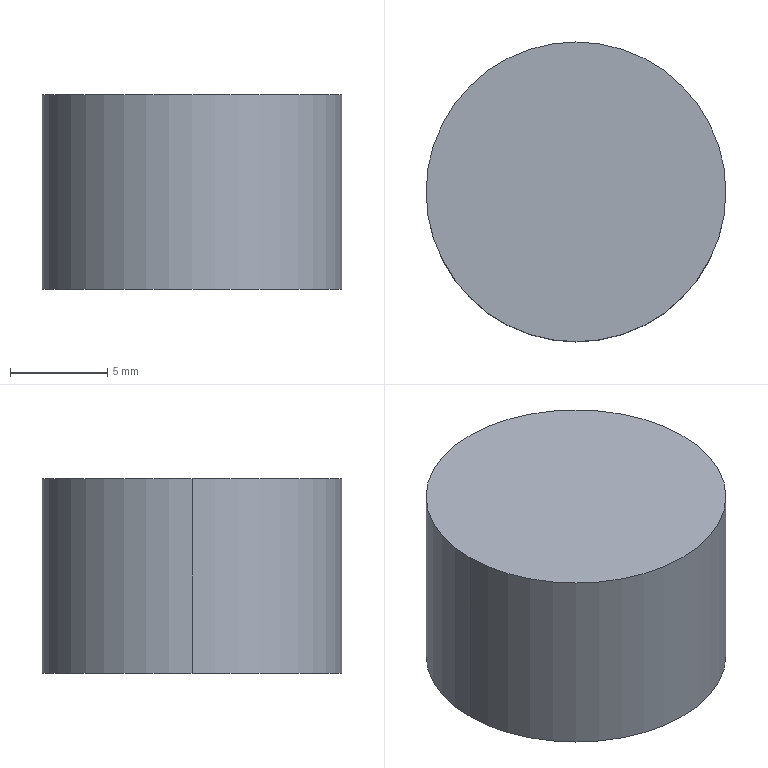Part | SolidWorks | features Extrusion 1 | 1 solid | 4 faces | box 15.395 x 15.395 x 10 mm | volume 1861 mm3 | cylinder 2 | plane 2 | commonest cylinder face diameters 15.395 x2
STEP:
#1=CARTESIAN_POINT('',(-9.358,0.,10.));
#2=VERTEX_POINT('',#1);
#3=CARTESIAN_POINT('',(-24.753,0.,10.));
#4=VERTEX_POINT('',#3);
#5=CARTESIAN_POINT('',(-17.056,0.,10.));
#6=DIRECTION('',(0.,0.,1.));
#7=DIRECTION('',(1.,0.,0.));
#8=AXIS2_PLACEMENT_3D('',#5,#6,#7);
#9=CIRCLE('',#8,7.697);
#10=EDGE_CURVE('',#2,#4,#9,.T.);
#11=ORIENTED_EDGE('',*,*,#10,.F.);
#12=CARTESIAN_POINT('',(-9.358,0.,0.));
#13=VERTEX_POINT('',#12);
#14=CARTESIAN_POINT('',(-9.358,0.,10.));
#15=DIRECTION('',(0.,0.,-1.));
#16=VECTOR('',#15,1000.);
#17=LINE('',#14,#16);
#18=EDGE_CURVE('',#2,#13,#17,.T.);
#19=ORIENTED_EDGE('',*,*,#18,.T.);
#20=CARTESIAN_POINT('',(-24.753,0.,0.));
#21=VERTEX_POINT('',#20);
#22=CARTESIAN_POINT('',(-17.056,0.,0.));
#23=DIRECTION('',(0.,0.,1.));
#24=DIRECTION('',(1.,0.,0.));
#25=AXIS2_PLACEMENT_3D('',#22,#23,#24);
#26=CIRCLE('',#25,7.697);
#27=EDGE_CURVE('',#13,#21,#26,.T.);
#28=ORIENTED_EDGE('',*,*,#27,.T.);
#29=CARTESIAN_POINT('',(-24.753,0.,10.));
#30=DIRECTION('',(0.,0.,-1.));
#31=VECTOR('',#30,1000.);
#32=LINE('',#29,#31);
#33=EDGE_CURVE('',#4,#21,#32,.T.);
#34=ORIENTED_EDGE('',*,*,#33,.F.);
#35=EDGE_LOOP('',(#11,#19,#28,#34));
#36=FACE_OUTER_BOUND('',#35,.T.);
#37=CARTESIAN_POINT('',(-17.056,0.,10.));
#38=DIRECTION('',(0.,0.,-1.));
#39=DIRECTION('',(-1.,0.,0.));
#40=AXIS2_PLACEMENT_3D('',#37,#38,#39);
#41=CYLINDRICAL_SURFACE('',#40,7.697);
#42=ADVANCED_FACE('',(#36),#41,.T.);
#43=ORIENTED_EDGE('',*,*,#18,.F.);
#44=CARTESIAN_POINT('',(-17.056,0.,10.));
#45=DIRECTION('',(0.,0.,1.));
#46=DIRECTION('',(1.,0.,0.));
#47=AXIS2_PLACEMENT_3D('',#44,#45,#46);
#48=CIRCLE('',#47,7.697);
#49=EDGE_CURVE('',#4,#2,#48,.T.);
#50=ORIENTED_EDGE('',*,*,#49,.F.);
#51=ORIENTED_EDGE('',*,*,#33,.T.);
#52=CARTESIAN_POINT('',(-17.056,0.,0.));
#53=DIRECTION('',(0.,0.,1.));
#54=DIRECTION('',(1.,0.,0.));
#55=AXIS2_PLACEMENT_3D('',#52,#53,#54);
#56=CIRCLE('',#55,7.697);
#57=EDGE_CURVE('',#21,#13,#56,.T.);
#58=ORIENTED_EDGE('',*,*,#57,.T.);
#59=EDGE_LOOP('',(#43,#50,#51,#58));
#60=FACE_OUTER_BOUND('',#59,.T.);
#61=CARTESIAN_POINT('',(-17.056,0.,10.));
#62=DIRECTION('',(0.,0.,-1.));
#63=DIRECTION('',(-1.,0.,0.));
#64=AXIS2_PLACEMENT_3D('',#61,#62,#63);
#65=CYLINDRICAL_SURFACE('',#64,7.697);
#66=ADVANCED_FACE('',(#60),#65,.T.);
#67=ORIENTED_EDGE('',*,*,#49,.T.);
#68=ORIENTED_EDGE('',*,*,#10,.T.);
#69=EDGE_LOOP('',(#67,#68));
#70=FACE_OUTER_BOUND('',#69,.T.);
#71=CARTESIAN_POINT('',(-17.056,0.,10.));
#72=DIRECTION('',(0.,0.,1.));
#73=DIRECTION('',(1.,0.,0.));
#74=AXIS2_PLACEMENT_3D('',#71,#72,#73);
#75=PLANE('',#74);
#76=ADVANCED_FACE('',(#70),#75,.T.);
#77=ORIENTED_EDGE('',*,*,#57,.F.);
#78=ORIENTED_EDGE('',*,*,#27,.F.);
#79=EDGE_LOOP('',(#77,#78));
#80=FACE_OUTER_BOUND('',#79,.T.);
#81=CARTESIAN_POINT('',(-17.056,0.,0.));
#82=DIRECTION('',(0.,0.,1.));
#83=DIRECTION('',(1.,0.,0.));
#84=AXIS2_PLACEMENT_3D('',#81,#82,#83);
#85=PLANE('',#84);
#86=ADVANCED_FACE('',(#80),#85,.F.);
#87=CLOSED_SHELL('',(#42,#66,#76,#86));
#88=MANIFOLD_SOLID_BREP('',#87);
#89=CARTESIAN_POINT('',(0.,0.,0.));
#90=DIRECTION('',(0.,0.,1.));
#91=DIRECTION('',(1.,0.,0.));
#92=AXIS2_PLACEMENT_3D('',#89,#90,#91);
#93=(LENGTH_UNIT()NAMED_UNIT(*)SI_UNIT(.MILLI.,.METRE.));
#94=UNCERTAINTY_MEASURE_WITH_UNIT(LENGTH_MEASURE(0.00001),#93,'','');
#95=(NAMED_UNIT(*)PLANE_ANGLE_UNIT()SI_UNIT($,.RADIAN.));
#96=(NAMED_UNIT(*)SI_UNIT($,.STERADIAN.)SOLID_ANGLE_UNIT());
#97=(GEOMETRIC_REPRESENTATION_CONTEXT(3)GLOBAL_UNCERTAINTY_ASSIGNED_CONTEXT((#94))GLOBAL_UNIT_ASSIGNED_CONTEXT((#93,#95,#96))REPRESENTATION_CONTEXT('',''));
#98=ADVANCED_BREP_SHAPE_REPRESENTATION('',(#88,#92),#97);